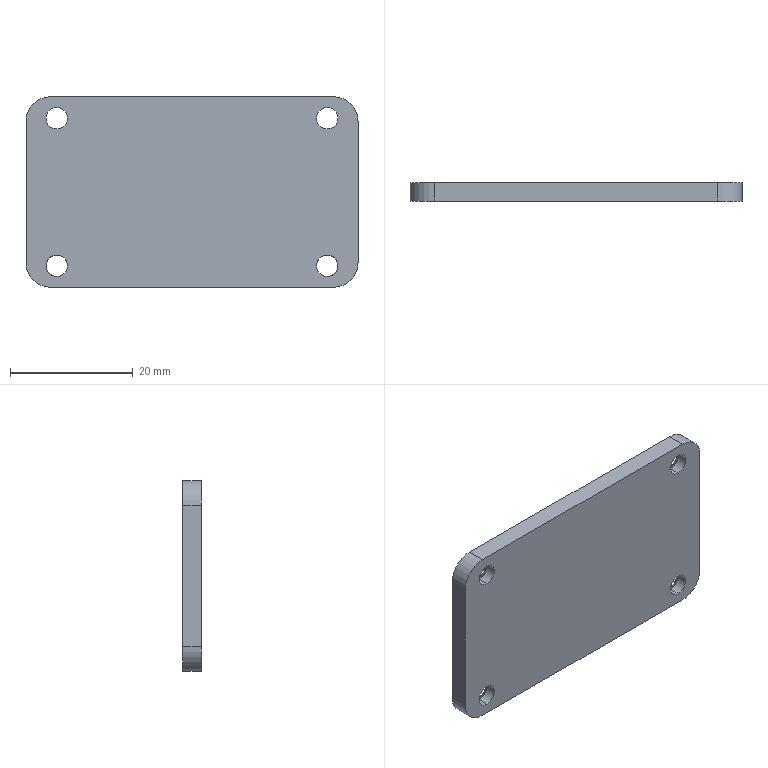Part | STEP file | 1 solid | 26 faces | box 54 x 3 x 31 mm | volume 4823 mm3 | cylinder 12 | cone 8 | plane 6 | commonest cylinder face diameters 3.5 x8 8 x4
STEP:
#1=CARTESIAN_POINT('',(-22.,1.75,13.75));
#2=VERTEX_POINT('',#1);
#3=CARTESIAN_POINT('',(-22.,1.75,10.25));
#4=VERTEX_POINT('',#3);
#5=CARTESIAN_POINT('',(-22.,1.75,12.));
#6=DIRECTION('',(0.,-1.,0.));
#7=DIRECTION('',(0.,0.,-1.));
#8=AXIS2_PLACEMENT_3D('',#5,#6,#7);
#9=CIRCLE('',#8,1.75);
#10=EDGE_CURVE('',#2,#4,#9,.T.);
#11=ORIENTED_EDGE('',*,*,#10,.F.);
#12=CARTESIAN_POINT('',(-22.,0.,13.75));
#13=VERTEX_POINT('',#12);
#14=CARTESIAN_POINT('',(-22.,9.585,13.75));
#15=DIRECTION('',(0.,-1.,0.));
#16=VECTOR('',#15,1000.);
#17=LINE('',#14,#16);
#18=EDGE_CURVE('',#2,#13,#17,.T.);
#19=ORIENTED_EDGE('',*,*,#18,.T.);
#20=CARTESIAN_POINT('',(-22.,0.,10.25));
#21=VERTEX_POINT('',#20);
#22=CARTESIAN_POINT('',(-22.,0.,12.));
#23=DIRECTION('',(0.,1.,0.));
#24=DIRECTION('',(0.,0.,-1.));
#25=AXIS2_PLACEMENT_3D('',#22,#23,#24);
#26=CIRCLE('',#25,1.75);
#27=EDGE_CURVE('',#21,#13,#26,.T.);
#28=ORIENTED_EDGE('',*,*,#27,.F.);
#29=CARTESIAN_POINT('',(-22.,9.585,10.25));
#30=DIRECTION('',(0.,-1.,0.));
#31=VECTOR('',#30,1000.);
#32=LINE('',#29,#31);
#33=EDGE_CURVE('',#4,#21,#32,.T.);
#34=ORIENTED_EDGE('',*,*,#33,.F.);
#35=EDGE_LOOP('',(#11,#19,#28,#34));
#36=FACE_OUTER_BOUND('',#35,.T.);
#37=CARTESIAN_POINT('',(-22.,9.585,12.));
#38=DIRECTION('',(0.,-1.,0.));
#39=DIRECTION('',(0.,0.,-1.));
#40=AXIS2_PLACEMENT_3D('',#37,#38,#39);
#41=CYLINDRICAL_SURFACE('',#40,1.75);
#42=ADVANCED_FACE('',(#36),#41,.F.);
#43=CARTESIAN_POINT('',(-22.,1.75,-10.25));
#44=VERTEX_POINT('',#43);
#45=CARTESIAN_POINT('',(-23.75,1.75,-12.));
#46=VERTEX_POINT('',#45);
#47=CARTESIAN_POINT('',(-22.,1.75,-12.));
#48=DIRECTION('',(0.,-1.,0.));
#49=DIRECTION('',(0.,0.,-1.));
#50=AXIS2_PLACEMENT_3D('',#47,#48,#49);
#51=CIRCLE('',#50,1.75);
#52=EDGE_CURVE('',#44,#46,#51,.T.);
#53=ORIENTED_EDGE('',*,*,#52,.F.);
#54=CARTESIAN_POINT('',(-22.,0.,-10.25));
#55=VERTEX_POINT('',#54);
#56=CARTESIAN_POINT('',(-22.,9.585,-10.25));
#57=DIRECTION('',(0.,-1.,0.));
#58=VECTOR('',#57,1000.);
#59=LINE('',#56,#58);
#60=EDGE_CURVE('',#44,#55,#59,.T.);
#61=ORIENTED_EDGE('',*,*,#60,.T.);
#62=CARTESIAN_POINT('',(-22.,0.,-13.75));
#63=VERTEX_POINT('',#62);
#64=CARTESIAN_POINT('',(-22.,0.,-12.));
#65=DIRECTION('',(0.,1.,0.));
#66=DIRECTION('',(0.,0.,-1.));
#67=AXIS2_PLACEMENT_3D('',#64,#65,#66);
#68=CIRCLE('',#67,1.75);
#69=EDGE_CURVE('',#63,#55,#68,.T.);
#70=ORIENTED_EDGE('',*,*,#69,.F.);
#71=CARTESIAN_POINT('',(-22.,1.75,-13.75));
#72=VERTEX_POINT('',#71);
#73=CARTESIAN_POINT('',(-22.,9.585,-13.75));
#74=DIRECTION('',(0.,-1.,0.));
#75=VECTOR('',#74,1000.);
#76=LINE('',#73,#75);
#77=EDGE_CURVE('',#72,#63,#76,.T.);
#78=ORIENTED_EDGE('',*,*,#77,.F.);
#79=CARTESIAN_POINT('',(-22.,1.75,-12.));
#80=DIRECTION('',(0.,-1.,0.));
#81=DIRECTION('',(0.,0.,-1.));
#82=AXIS2_PLACEMENT_3D('',#79,#80,#81);
#83=CIRCLE('',#82,1.75);
#84=EDGE_CURVE('',#46,#72,#83,.T.);
#85=ORIENTED_EDGE('',*,*,#84,.F.);
#86=EDGE_LOOP('',(#53,#61,#70,#78,#85));
#87=FACE_OUTER_BOUND('',#86,.T.);
#88=CARTESIAN_POINT('',(-22.,9.585,-12.));
#89=DIRECTION('',(0.,-1.,0.));
#90=DIRECTION('',(0.,0.,-1.));
#91=AXIS2_PLACEMENT_3D('',#88,#89,#90);
#92=CYLINDRICAL_SURFACE('',#91,1.75);
#93=ADVANCED_FACE('',(#87),#92,.F.);
#94=CARTESIAN_POINT('',(22.,1.75,-10.25));
#95=VERTEX_POINT('',#94);
#96=CARTESIAN_POINT('',(20.25,1.75,-12.));
#97=VERTEX_POINT('',#96);
#98=CARTESIAN_POINT('',(22.,1.75,-12.));
#99=DIRECTION('',(0.,-1.,0.));
#100=DIRECTION('',(0.,0.,-1.));
#101=AXIS2_PLACEMENT_3D('',#98,#99,#100);
#102=CIRCLE('',#101,1.75);
#103=EDGE_CURVE('',#95,#97,#102,.T.);
#104=ORIENTED_EDGE('',*,*,#103,.F.);
#105=CARTESIAN_POINT('',(22.,0.,-10.25));
#106=VERTEX_POINT('',#105);
#107=CARTESIAN_POINT('',(22.,9.585,-10.25));
#108=DIRECTION('',(0.,-1.,0.));
#109=VECTOR('',#108,1000.);
#110=LINE('',#107,#109);
#111=EDGE_CURVE('',#95,#106,#110,.T.);
#112=ORIENTED_EDGE('',*,*,#111,.T.);
#113=CARTESIAN_POINT('',(22.,0.,-13.75));
#114=VERTEX_POINT('',#113);
#115=CARTESIAN_POINT('',(22.,0.,-12.));
#116=DIRECTION('',(0.,1.,0.));
#117=DIRECTION('',(0.,0.,-1.));
#118=AXIS2_PLACEMENT_3D('',#115,#116,#117);
#119=CIRCLE('',#118,1.75);
#120=EDGE_CURVE('',#114,#106,#119,.T.);
#121=ORIENTED_EDGE('',*,*,#120,.F.);
#122=CARTESIAN_POINT('',(22.,1.75,-13.75));
#123=VERTEX_POINT('',#122);
#124=CARTESIAN_POINT('',(22.,9.585,-13.75));
#125=DIRECTION('',(0.,-1.,0.));
#126=VECTOR('',#125,1000.);
#127=LINE('',#124,#126);
#128=EDGE_CURVE('',#123,#114,#127,.T.);
#129=ORIENTED_EDGE('',*,*,#128,.F.);
#130=CARTESIAN_POINT('',(22.,1.75,-12.));
#131=DIRECTION('',(0.,-1.,0.));
#132=DIRECTION('',(0.,0.,-1.));
#133=AXIS2_PLACEMENT_3D('',#130,#131,#132);
#134=CIRCLE('',#133,1.75);
#135=EDGE_CURVE('',#97,#123,#134,.T.);
#136=ORIENTED_EDGE('',*,*,#135,.F.);
#137=EDGE_LOOP('',(#104,#112,#121,#129,#136));
#138=FACE_OUTER_BOUND('',#137,.T.);
#139=CARTESIAN_POINT('',(22.,9.585,-12.));
#140=DIRECTION('',(0.,-1.,0.));
#141=DIRECTION('',(0.,0.,-1.));
#142=AXIS2_PLACEMENT_3D('',#139,#140,#141);
#143=CYLINDRICAL_SURFACE('',#142,1.75);
#144=ADVANCED_FACE('',(#138),#143,.F.);
#145=CARTESIAN_POINT('',(22.,1.75,13.75));
#146=VERTEX_POINT('',#145);
#147=CARTESIAN_POINT('',(22.,1.75,10.25));
#148=VERTEX_POINT('',#147);
#149=CARTESIAN_POINT('',(22.,1.75,12.));
#150=DIRECTION('',(0.,-1.,0.));
#151=DIRECTION('',(0.,0.,-1.));
#152=AXIS2_PLACEMENT_3D('',#149,#150,#151);
#153=CIRCLE('',#152,1.75);
#154=EDGE_CURVE('',#146,#148,#153,.T.);
#155=ORIENTED_EDGE('',*,*,#154,.F.);
#156=CARTESIAN_POINT('',(22.,0.,13.75));
#157=VERTEX_POINT('',#156);
#158=CARTESIAN_POINT('',(22.,9.585,13.75));
#159=DIRECTION('',(0.,-1.,0.));
#160=VECTOR('',#159,1000.);
#161=LINE('',#158,#160);
#162=EDGE_CURVE('',#146,#157,#161,.T.);
#163=ORIENTED_EDGE('',*,*,#162,.T.);
#164=CARTESIAN_POINT('',(22.,0.,10.25));
#165=VERTEX_POINT('',#164);
#166=CARTESIAN_POINT('',(22.,0.,12.));
#167=DIRECTION('',(0.,1.,0.));
#168=DIRECTION('',(0.,0.,-1.));
#169=AXIS2_PLACEMENT_3D('',#166,#167,#168);
#170=CIRCLE('',#169,1.75);
#171=EDGE_CURVE('',#165,#157,#170,.T.);
#172=ORIENTED_EDGE('',*,*,#171,.F.);
#173=CARTESIAN_POINT('',(22.,9.585,10.25));
#174=DIRECTION('',(0.,-1.,0.));
#175=VECTOR('',#174,1000.);
#176=LINE('',#173,#175);
#177=EDGE_CURVE('',#148,#165,#176,.T.);
#178=ORIENTED_EDGE('',*,*,#177,.F.);
#179=EDGE_LOOP('',(#155,#163,#172,#178));
#180=FACE_OUTER_BOUND('',#179,.T.);
#181=CARTESIAN_POINT('',(22.,9.585,12.));
#182=DIRECTION('',(0.,-1.,0.));
#183=DIRECTION('',(0.,0.,-1.));
#184=AXIS2_PLACEMENT_3D('',#181,#182,#183);
#185=CYLINDRICAL_SURFACE('',#184,1.75);
#186=ADVANCED_FACE('',(#180),#185,.F.);
#187=ORIENTED_EDGE('',*,*,#10,.T.);
#188=CARTESIAN_POINT('',(-22.,3.,9.));
#189=VERTEX_POINT('',#188);
#190=CARTESIAN_POINT('',(-22.,3.,9.));
#191=DIRECTION('',(0.,0.7071,-0.7071));
#192=VECTOR('',#191,1000.);
#193=LINE('',#190,#192);
#194=EDGE_CURVE('',#4,#189,#193,.T.);
#195=ORIENTED_EDGE('',*,*,#194,.T.);
#196=CARTESIAN_POINT('',(-22.,3.,15.));
#197=VERTEX_POINT('',#196);
#198=CARTESIAN_POINT('',(-22.,3.,12.));
#199=DIRECTION('',(0.,-1.,0.));
#200=DIRECTION('',(0.,0.,1.));
#201=AXIS2_PLACEMENT_3D('',#198,#199,#200);
#202=CIRCLE('',#201,3.);
#203=EDGE_CURVE('',#197,#189,#202,.T.);
#204=ORIENTED_EDGE('',*,*,#203,.F.);
#205=CARTESIAN_POINT('',(-22.,3.,15.));
#206=DIRECTION('',(0.,0.7071,0.7071));
#207=VECTOR('',#206,1000.);
#208=LINE('',#205,#207);
#209=EDGE_CURVE('',#2,#197,#208,.T.);
#210=ORIENTED_EDGE('',*,*,#209,.F.);
#211=EDGE_LOOP('',(#187,#195,#204,#210));
#212=FACE_OUTER_BOUND('',#211,.T.);
#213=CARTESIAN_POINT('',(-22.,3.,12.));
#214=DIRECTION('',(0.,1.,0.));
#215=DIRECTION('',(0.,0.,1.));
#216=AXIS2_PLACEMENT_3D('',#213,#214,#215);
#217=CONICAL_SURFACE('',#216,3.,0.7854);
#218=ADVANCED_FACE('',(#212),#217,.F.);
#219=ORIENTED_EDGE('',*,*,#84,.T.);
#220=CARTESIAN_POINT('',(-20.25,1.75,-12.));
#221=VERTEX_POINT('',#220);
#222=CARTESIAN_POINT('',(-22.,1.75,-12.));
#223=DIRECTION('',(0.,-1.,0.));
#224=DIRECTION('',(0.,0.,-1.));
#225=AXIS2_PLACEMENT_3D('',#222,#223,#224);
#226=CIRCLE('',#225,1.75);
#227=EDGE_CURVE('',#72,#221,#226,.T.);
#228=ORIENTED_EDGE('',*,*,#227,.T.);
#229=CARTESIAN_POINT('',(-19.,3.,-12.));
#230=VERTEX_POINT('',#229);
#231=CARTESIAN_POINT('',(-19.,3.,-12.));
#232=DIRECTION('',(0.7071,0.7071,0.));
#233=VECTOR('',#232,1000.);
#234=LINE('',#231,#233);
#235=EDGE_CURVE('',#221,#230,#234,.T.);
#236=ORIENTED_EDGE('',*,*,#235,.T.);
#237=CARTESIAN_POINT('',(-25.,3.,-12.));
#238=VERTEX_POINT('',#237);
#239=CARTESIAN_POINT('',(-22.,3.,-12.));
#240=DIRECTION('',(0.,-1.,0.));
#241=DIRECTION('',(-1.,0.,0.));
#242=AXIS2_PLACEMENT_3D('',#239,#240,#241);
#243=CIRCLE('',#242,3.);
#244=EDGE_CURVE('',#238,#230,#243,.T.);
#245=ORIENTED_EDGE('',*,*,#244,.F.);
#246=CARTESIAN_POINT('',(-25.,3.,-12.));
#247=DIRECTION('',(-0.7071,0.7071,0.));
#248=VECTOR('',#247,1000.);
#249=LINE('',#246,#248);
#250=EDGE_CURVE('',#46,#238,#249,.T.);
#251=ORIENTED_EDGE('',*,*,#250,.F.);
#252=EDGE_LOOP('',(#219,#228,#236,#245,#251));
#253=FACE_OUTER_BOUND('',#252,.T.);
#254=CARTESIAN_POINT('',(-22.,3.,-12.));
#255=DIRECTION('',(0.,1.,0.));
#256=DIRECTION('',(-1.,0.,0.));
#257=AXIS2_PLACEMENT_3D('',#254,#255,#256);
#258=CONICAL_SURFACE('',#257,3.,0.7854);
#259=ADVANCED_FACE('',(#253),#258,.F.);
#260=ORIENTED_EDGE('',*,*,#135,.T.);
#261=CARTESIAN_POINT('',(23.75,1.75,-12.));
#262=VERTEX_POINT('',#261);
#263=CARTESIAN_POINT('',(22.,1.75,-12.));
#264=DIRECTION('',(0.,-1.,0.));
#265=DIRECTION('',(0.,0.,-1.));
#266=AXIS2_PLACEMENT_3D('',#263,#264,#265);
#267=CIRCLE('',#266,1.75);
#268=EDGE_CURVE('',#123,#262,#267,.T.);
#269=ORIENTED_EDGE('',*,*,#268,.T.);
#270=CARTESIAN_POINT('',(25.,3.,-12.));
#271=VERTEX_POINT('',#270);
#272=CARTESIAN_POINT('',(25.,3.,-12.));
#273=DIRECTION('',(0.7071,0.7071,0.));
#274=VECTOR('',#273,1000.);
#275=LINE('',#272,#274);
#276=EDGE_CURVE('',#262,#271,#275,.T.);
#277=ORIENTED_EDGE('',*,*,#276,.T.);
#278=CARTESIAN_POINT('',(19.,3.,-12.));
#279=VERTEX_POINT('',#278);
#280=CARTESIAN_POINT('',(22.,3.,-12.));
#281=DIRECTION('',(0.,-1.,0.));
#282=DIRECTION('',(-1.,0.,0.));
#283=AXIS2_PLACEMENT_3D('',#280,#281,#282);
#284=CIRCLE('',#283,3.);
#285=EDGE_CURVE('',#279,#271,#284,.T.);
#286=ORIENTED_EDGE('',*,*,#285,.F.);
#287=CARTESIAN_POINT('',(19.,3.,-12.));
#288=DIRECTION('',(-0.7071,0.7071,0.));
#289=VECTOR('',#288,1000.);
#290=LINE('',#287,#289);
#291=EDGE_CURVE('',#97,#279,#290,.T.);
#292=ORIENTED_EDGE('',*,*,#291,.F.);
#293=EDGE_LOOP('',(#260,#269,#277,#286,#292));
#294=FACE_OUTER_BOUND('',#293,.T.);
#295=CARTESIAN_POINT('',(22.,3.,-12.));
#296=DIRECTION('',(0.,1.,0.));
#297=DIRECTION('',(-1.,0.,0.));
#298=AXIS2_PLACEMENT_3D('',#295,#296,#297);
#299=CONICAL_SURFACE('',#298,3.,0.7854);
#300=ADVANCED_FACE('',(#294),#299,.F.);
#301=ORIENTED_EDGE('',*,*,#154,.T.);
#302=CARTESIAN_POINT('',(22.,3.,9.));
#303=VERTEX_POINT('',#302);
#304=CARTESIAN_POINT('',(22.,3.,9.));
#305=DIRECTION('',(0.,0.7071,-0.7071));
#306=VECTOR('',#305,1000.);
#307=LINE('',#304,#306);
#308=EDGE_CURVE('',#148,#303,#307,.T.);
#309=ORIENTED_EDGE('',*,*,#308,.T.);
#310=CARTESIAN_POINT('',(22.,3.,15.));
#311=VERTEX_POINT('',#310);
#312=CARTESIAN_POINT('',(22.,3.,12.));
#313=DIRECTION('',(0.,-1.,0.));
#314=DIRECTION('',(0.,0.,1.));
#315=AXIS2_PLACEMENT_3D('',#312,#313,#314);
#316=CIRCLE('',#315,3.);
#317=EDGE_CURVE('',#311,#303,#316,.T.);
#318=ORIENTED_EDGE('',*,*,#317,.F.);
#319=CARTESIAN_POINT('',(22.,3.,15.));
#320=DIRECTION('',(0.,0.7071,0.7071));
#321=VECTOR('',#320,1000.);
#322=LINE('',#319,#321);
#323=EDGE_CURVE('',#146,#311,#322,.T.);
#324=ORIENTED_EDGE('',*,*,#323,.F.);
#325=EDGE_LOOP('',(#301,#309,#318,#324));
#326=FACE_OUTER_BOUND('',#325,.T.);
#327=CARTESIAN_POINT('',(22.,3.,12.));
#328=DIRECTION('',(0.,1.,0.));
#329=DIRECTION('',(0.,0.,1.));
#330=AXIS2_PLACEMENT_3D('',#327,#328,#329);
#331=CONICAL_SURFACE('',#330,3.,0.7854);
#332=ADVANCED_FACE('',(#326),#331,.F.);
#333=CARTESIAN_POINT('',(23.,0.,-15.5));
#334=VERTEX_POINT('',#333);
#335=CARTESIAN_POINT('',(27.,0.,-11.5));
#336=VERTEX_POINT('',#335);
#337=CARTESIAN_POINT('',(23.,0.,-11.5));
#338=DIRECTION('',(0.,-1.,0.));
#339=DIRECTION('',(0.,0.,-1.));
#340=AXIS2_PLACEMENT_3D('',#337,#338,#339);
#341=CIRCLE('',#340,4.);
#342=EDGE_CURVE('',#334,#336,#341,.T.);
#343=ORIENTED_EDGE('',*,*,#342,.T.);
#344=CARTESIAN_POINT('',(27.,0.,11.5));
#345=VERTEX_POINT('',#344);
#346=CARTESIAN_POINT('',(27.,0.,-62.266));
#347=DIRECTION('',(0.,0.,1.));
#348=VECTOR('',#347,1000.);
#349=LINE('',#346,#348);
#350=EDGE_CURVE('',#336,#345,#349,.T.);
#351=ORIENTED_EDGE('',*,*,#350,.T.);
#352=CARTESIAN_POINT('',(23.,0.,15.5));
#353=VERTEX_POINT('',#352);
#354=CARTESIAN_POINT('',(23.,0.,11.5));
#355=DIRECTION('',(0.,-1.,0.));
#356=DIRECTION('',(0.,0.,-1.));
#357=AXIS2_PLACEMENT_3D('',#354,#355,#356);
#358=CIRCLE('',#357,4.);
#359=EDGE_CURVE('',#345,#353,#358,.T.);
#360=ORIENTED_EDGE('',*,*,#359,.T.);
#361=CARTESIAN_POINT('',(-23.,0.,15.5));
#362=VERTEX_POINT('',#361);
#363=CARTESIAN_POINT('',(62.266,0.,15.5));
#364=DIRECTION('',(-1.,0.,0.));
#365=VECTOR('',#364,1000.);
#366=LINE('',#363,#365);
#367=EDGE_CURVE('',#353,#362,#366,.T.);
#368=ORIENTED_EDGE('',*,*,#367,.T.);
#369=CARTESIAN_POINT('',(-27.,0.,11.5));
#370=VERTEX_POINT('',#369);
#371=CARTESIAN_POINT('',(-23.,0.,11.5));
#372=DIRECTION('',(0.,-1.,0.));
#373=DIRECTION('',(0.,0.,-1.));
#374=AXIS2_PLACEMENT_3D('',#371,#372,#373);
#375=CIRCLE('',#374,4.);
#376=EDGE_CURVE('',#362,#370,#375,.T.);
#377=ORIENTED_EDGE('',*,*,#376,.T.);
#378=CARTESIAN_POINT('',(-27.,0.,-11.5));
#379=VERTEX_POINT('',#378);
#380=CARTESIAN_POINT('',(-27.,0.,-62.266));
#381=DIRECTION('',(0.,0.,-1.));
#382=VECTOR('',#381,1000.);
#383=LINE('',#380,#382);
#384=EDGE_CURVE('',#370,#379,#383,.T.);
#385=ORIENTED_EDGE('',*,*,#384,.T.);
#386=CARTESIAN_POINT('',(-23.,0.,-15.5));
#387=VERTEX_POINT('',#386);
#388=CARTESIAN_POINT('',(-23.,0.,-11.5));
#389=DIRECTION('',(0.,-1.,0.));
#390=DIRECTION('',(0.,0.,-1.));
#391=AXIS2_PLACEMENT_3D('',#388,#389,#390);
#392=CIRCLE('',#391,4.);
#393=EDGE_CURVE('',#379,#387,#392,.T.);
#394=ORIENTED_EDGE('',*,*,#393,.T.);
#395=CARTESIAN_POINT('',(62.266,0.,-15.5));
#396=DIRECTION('',(1.,0.,0.));
#397=VECTOR('',#396,1000.);
#398=LINE('',#395,#397);
#399=EDGE_CURVE('',#387,#334,#398,.T.);
#400=ORIENTED_EDGE('',*,*,#399,.T.);
#401=EDGE_LOOP('',(#343,#351,#360,#368,#377,#385,#394,#400));
#402=FACE_OUTER_BOUND('',#401,.T.);
#403=ORIENTED_EDGE('',*,*,#27,.T.);
#404=CARTESIAN_POINT('',(-22.,0.,12.));
#405=DIRECTION('',(0.,1.,0.));
#406=DIRECTION('',(0.,0.,-1.));
#407=AXIS2_PLACEMENT_3D('',#404,#405,#406);
#408=CIRCLE('',#407,1.75);
#409=EDGE_CURVE('',#13,#21,#408,.T.);
#410=ORIENTED_EDGE('',*,*,#409,.T.);
#411=EDGE_LOOP('',(#403,#410));
#412=FACE_BOUND('',#411,.T.);
#413=ORIENTED_EDGE('',*,*,#69,.T.);
#414=CARTESIAN_POINT('',(-22.,0.,-12.));
#415=DIRECTION('',(0.,1.,0.));
#416=DIRECTION('',(0.,0.,-1.));
#417=AXIS2_PLACEMENT_3D('',#414,#415,#416);
#418=CIRCLE('',#417,1.75);
#419=EDGE_CURVE('',#55,#63,#418,.T.);
#420=ORIENTED_EDGE('',*,*,#419,.T.);
#421=EDGE_LOOP('',(#413,#420));
#422=FACE_BOUND('',#421,.T.);
#423=ORIENTED_EDGE('',*,*,#120,.T.);
#424=CARTESIAN_POINT('',(22.,0.,-12.));
#425=DIRECTION('',(0.,1.,0.));
#426=DIRECTION('',(0.,0.,-1.));
#427=AXIS2_PLACEMENT_3D('',#424,#425,#426);
#428=CIRCLE('',#427,1.75);
#429=EDGE_CURVE('',#106,#114,#428,.T.);
#430=ORIENTED_EDGE('',*,*,#429,.T.);
#431=EDGE_LOOP('',(#423,#430));
#432=FACE_BOUND('',#431,.T.);
#433=ORIENTED_EDGE('',*,*,#171,.T.);
#434=CARTESIAN_POINT('',(22.,0.,12.));
#435=DIRECTION('',(0.,1.,0.));
#436=DIRECTION('',(0.,0.,-1.));
#437=AXIS2_PLACEMENT_3D('',#434,#435,#436);
#438=CIRCLE('',#437,1.75);
#439=EDGE_CURVE('',#157,#165,#438,.T.);
#440=ORIENTED_EDGE('',*,*,#439,.T.);
#441=EDGE_LOOP('',(#433,#440));
#442=FACE_BOUND('',#441,.T.);
#443=CARTESIAN_POINT('',(62.266,0.,-62.266));
#444=DIRECTION('',(0.,-1.,0.));
#445=DIRECTION('',(0.,0.,-1.));
#446=AXIS2_PLACEMENT_3D('',#443,#444,#445);
#447=PLANE('',#446);
#448=ADVANCED_FACE('',(#402,#412,#422,#432,#442),#447,.T.);
#449=CARTESIAN_POINT('',(27.,3.,-11.5));
#450=VERTEX_POINT('',#449);
#451=CARTESIAN_POINT('',(27.,41.767,-11.5));
#452=DIRECTION('',(0.,1.,0.));
#453=VECTOR('',#452,1000.);
#454=LINE('',#451,#453);
#455=EDGE_CURVE('',#336,#450,#454,.T.);
#456=ORIENTED_EDGE('',*,*,#455,.T.);
#457=CARTESIAN_POINT('',(27.,3.,11.5));
#458=VERTEX_POINT('',#457);
#459=CARTESIAN_POINT('',(27.,3.,-54.267));
#460=DIRECTION('',(0.,0.,1.));
#461=VECTOR('',#460,1000.);
#462=LINE('',#459,#461);
#463=EDGE_CURVE('',#450,#458,#462,.T.);
#464=ORIENTED_EDGE('',*,*,#463,.T.);
#465=CARTESIAN_POINT('',(27.,41.767,11.5));
#466=DIRECTION('',(0.,-1.,0.));
#467=VECTOR('',#466,1000.);
#468=LINE('',#465,#467);
#469=EDGE_CURVE('',#458,#345,#468,.T.);
#470=ORIENTED_EDGE('',*,*,#469,.T.);
#471=ORIENTED_EDGE('',*,*,#350,.F.);
#472=EDGE_LOOP('',(#456,#464,#470,#471));
#473=FACE_OUTER_BOUND('',#472,.T.);
#474=CARTESIAN_POINT('',(27.,41.767,-54.267));
#475=DIRECTION('',(1.,0.,0.));
#476=DIRECTION('',(0.,1.,0.));
#477=AXIS2_PLACEMENT_3D('',#474,#475,#476);
#478=PLANE('',#477);
#479=ADVANCED_FACE('',(#473),#478,.T.);
#480=ORIENTED_EDGE('',*,*,#342,.F.);
#481=CARTESIAN_POINT('',(23.,3.,-15.5));
#482=VERTEX_POINT('',#481);
#483=CARTESIAN_POINT('',(23.,12.605,-15.5));
#484=DIRECTION('',(0.,1.,0.));
#485=VECTOR('',#484,1000.);
#486=LINE('',#483,#485);
#487=EDGE_CURVE('',#334,#482,#486,.T.);
#488=ORIENTED_EDGE('',*,*,#487,.T.);
#489=CARTESIAN_POINT('',(23.,3.,-11.5));
#490=DIRECTION('',(0.,-1.,0.));
#491=DIRECTION('',(0.,0.,-1.));
#492=AXIS2_PLACEMENT_3D('',#489,#490,#491);
#493=CIRCLE('',#492,4.);
#494=EDGE_CURVE('',#482,#450,#493,.T.);
#495=ORIENTED_EDGE('',*,*,#494,.T.);
#496=ORIENTED_EDGE('',*,*,#455,.F.);
#497=EDGE_LOOP('',(#480,#488,#495,#496));
#498=FACE_OUTER_BOUND('',#497,.T.);
#499=CARTESIAN_POINT('',(23.,12.605,-11.5));
#500=DIRECTION('',(0.,-1.,0.));
#501=DIRECTION('',(0.,0.,-1.));
#502=AXIS2_PLACEMENT_3D('',#499,#500,#501);
#503=CYLINDRICAL_SURFACE('',#502,4.);
#504=ADVANCED_FACE('',(#498),#503,.T.);
#505=CARTESIAN_POINT('',(-23.,3.,-15.5));
#506=VERTEX_POINT('',#505);
#507=CARTESIAN_POINT('',(-23.,76.139,-15.5));
#508=DIRECTION('',(0.,1.,0.));
#509=VECTOR('',#508,1000.);
#510=LINE('',#507,#509);
#511=EDGE_CURVE('',#387,#506,#510,.T.);
#512=ORIENTED_EDGE('',*,*,#511,.T.);
#513=CARTESIAN_POINT('',(-100.139,3.,-15.5));
#514=DIRECTION('',(1.,0.,0.));
#515=VECTOR('',#514,1000.);
#516=LINE('',#513,#515);
#517=EDGE_CURVE('',#506,#482,#516,.T.);
#518=ORIENTED_EDGE('',*,*,#517,.T.);
#519=ORIENTED_EDGE('',*,*,#487,.F.);
#520=ORIENTED_EDGE('',*,*,#399,.F.);
#521=EDGE_LOOP('',(#512,#518,#519,#520));
#522=FACE_OUTER_BOUND('',#521,.T.);
#523=CARTESIAN_POINT('',(-100.139,76.139,-15.5));
#524=DIRECTION('',(0.,0.,-1.));
#525=DIRECTION('',(0.,-1.,0.));
#526=AXIS2_PLACEMENT_3D('',#523,#524,#525);
#527=PLANE('',#526);
#528=ADVANCED_FACE('',(#522),#527,.T.);
#529=ORIENTED_EDGE('',*,*,#393,.F.);
#530=CARTESIAN_POINT('',(-27.,3.,-11.5));
#531=VERTEX_POINT('',#530);
#532=CARTESIAN_POINT('',(-27.,12.605,-11.5));
#533=DIRECTION('',(0.,1.,0.));
#534=VECTOR('',#533,1000.);
#535=LINE('',#532,#534);
#536=EDGE_CURVE('',#379,#531,#535,.T.);
#537=ORIENTED_EDGE('',*,*,#536,.T.);
#538=CARTESIAN_POINT('',(-23.,3.,-11.5));
#539=DIRECTION('',(0.,-1.,0.));
#540=DIRECTION('',(0.,0.,-1.));
#541=AXIS2_PLACEMENT_3D('',#538,#539,#540);
#542=CIRCLE('',#541,4.);
#543=EDGE_CURVE('',#531,#506,#542,.T.);
#544=ORIENTED_EDGE('',*,*,#543,.T.);
#545=ORIENTED_EDGE('',*,*,#511,.F.);
#546=EDGE_LOOP('',(#529,#537,#544,#545));
#547=FACE_OUTER_BOUND('',#546,.T.);
#548=CARTESIAN_POINT('',(-23.,12.605,-11.5));
#549=DIRECTION('',(0.,-1.,0.));
#550=DIRECTION('',(0.,0.,-1.));
#551=AXIS2_PLACEMENT_3D('',#548,#549,#550);
#552=CYLINDRICAL_SURFACE('',#551,4.);
#553=ADVANCED_FACE('',(#547),#552,.T.);
#554=CARTESIAN_POINT('',(-27.,3.,11.5));
#555=VERTEX_POINT('',#554);
#556=CARTESIAN_POINT('',(-27.,41.767,11.5));
#557=DIRECTION('',(0.,1.,0.));
#558=VECTOR('',#557,1000.);
#559=LINE('',#556,#558);
#560=EDGE_CURVE('',#370,#555,#559,.T.);
#561=ORIENTED_EDGE('',*,*,#560,.T.);
#562=CARTESIAN_POINT('',(-27.,3.,23.267));
#563=DIRECTION('',(0.,0.,-1.));
#564=VECTOR('',#563,1000.);
#565=LINE('',#562,#564);
#566=EDGE_CURVE('',#555,#531,#565,.T.);
#567=ORIENTED_EDGE('',*,*,#566,.T.);
#568=ORIENTED_EDGE('',*,*,#536,.F.);
#569=ORIENTED_EDGE('',*,*,#384,.F.);
#570=EDGE_LOOP('',(#561,#567,#568,#569));
#571=FACE_OUTER_BOUND('',#570,.T.);
#572=CARTESIAN_POINT('',(-27.,41.767,23.267));
#573=DIRECTION('',(-1.,0.,0.));
#574=DIRECTION('',(0.,0.,1.));
#575=AXIS2_PLACEMENT_3D('',#572,#573,#574);
#576=PLANE('',#575);
#577=ADVANCED_FACE('',(#571),#576,.T.);
#578=ORIENTED_EDGE('',*,*,#376,.F.);
#579=CARTESIAN_POINT('',(-23.,3.,15.5));
#580=VERTEX_POINT('',#579);
#581=CARTESIAN_POINT('',(-23.,12.605,15.5));
#582=DIRECTION('',(0.,1.,0.));
#583=VECTOR('',#582,1000.);
#584=LINE('',#581,#583);
#585=EDGE_CURVE('',#362,#580,#584,.T.);
#586=ORIENTED_EDGE('',*,*,#585,.T.);
#587=CARTESIAN_POINT('',(-23.,3.,11.5));
#588=DIRECTION('',(0.,-1.,0.));
#589=DIRECTION('',(0.,0.,-1.));
#590=AXIS2_PLACEMENT_3D('',#587,#588,#589);
#591=CIRCLE('',#590,4.);
#592=EDGE_CURVE('',#580,#555,#591,.T.);
#593=ORIENTED_EDGE('',*,*,#592,.T.);
#594=ORIENTED_EDGE('',*,*,#560,.F.);
#595=EDGE_LOOP('',(#578,#586,#593,#594));
#596=FACE_OUTER_BOUND('',#595,.T.);
#597=CARTESIAN_POINT('',(-23.,12.605,11.5));
#598=DIRECTION('',(0.,-1.,0.));
#599=DIRECTION('',(0.,0.,-1.));
#600=AXIS2_PLACEMENT_3D('',#597,#598,#599);
#601=CYLINDRICAL_SURFACE('',#600,4.);
#602=ADVANCED_FACE('',(#596),#601,.T.);
#603=ORIENTED_EDGE('',*,*,#585,.F.);
#604=ORIENTED_EDGE('',*,*,#367,.F.);
#605=CARTESIAN_POINT('',(23.,3.,15.5));
#606=VERTEX_POINT('',#605);
#607=CARTESIAN_POINT('',(23.,76.139,15.5));
#608=DIRECTION('',(0.,1.,0.));
#609=VECTOR('',#608,1000.);
#610=LINE('',#607,#609);
#611=EDGE_CURVE('',#353,#606,#610,.T.);
#612=ORIENTED_EDGE('',*,*,#611,.T.);
#613=CARTESIAN_POINT('',(46.139,3.,15.5));
#614=DIRECTION('',(-1.,0.,0.));
#615=VECTOR('',#614,1000.);
#616=LINE('',#613,#615);
#617=EDGE_CURVE('',#606,#580,#616,.T.);
#618=ORIENTED_EDGE('',*,*,#617,.T.);
#619=EDGE_LOOP('',(#603,#604,#612,#618));
#620=FACE_OUTER_BOUND('',#619,.T.);
#621=CARTESIAN_POINT('',(46.139,76.139,15.5));
#622=DIRECTION('',(0.,0.,1.));
#623=DIRECTION('',(1.,0.,0.));
#624=AXIS2_PLACEMENT_3D('',#621,#622,#623);
#625=PLANE('',#624);
#626=ADVANCED_FACE('',(#620),#625,.T.);
#627=ORIENTED_EDGE('',*,*,#359,.F.);
#628=ORIENTED_EDGE('',*,*,#469,.F.);
#629=CARTESIAN_POINT('',(23.,3.,11.5));
#630=DIRECTION('',(0.,-1.,0.));
#631=DIRECTION('',(0.,0.,-1.));
#632=AXIS2_PLACEMENT_3D('',#629,#630,#631);
#633=CIRCLE('',#632,4.);
#634=EDGE_CURVE('',#458,#606,#633,.T.);
#635=ORIENTED_EDGE('',*,*,#634,.T.);
#636=ORIENTED_EDGE('',*,*,#611,.F.);
#637=EDGE_LOOP('',(#627,#628,#635,#636));
#638=FACE_OUTER_BOUND('',#637,.T.);
#639=CARTESIAN_POINT('',(23.,12.605,11.5));
#640=DIRECTION('',(0.,-1.,0.));
#641=DIRECTION('',(0.,0.,-1.));
#642=AXIS2_PLACEMENT_3D('',#639,#640,#641);
#643=CYLINDRICAL_SURFACE('',#642,4.);
#644=ADVANCED_FACE('',(#638),#643,.T.);
#645=ORIENTED_EDGE('',*,*,#18,.F.);
#646=CARTESIAN_POINT('',(-22.,1.75,12.));
#647=DIRECTION('',(0.,-1.,0.));
#648=DIRECTION('',(0.,0.,-1.));
#649=AXIS2_PLACEMENT_3D('',#646,#647,#648);
#650=CIRCLE('',#649,1.75);
#651=EDGE_CURVE('',#4,#2,#650,.T.);
#652=ORIENTED_EDGE('',*,*,#651,.F.);
#653=ORIENTED_EDGE('',*,*,#33,.T.);
#654=ORIENTED_EDGE('',*,*,#409,.F.);
#655=EDGE_LOOP('',(#645,#652,#653,#654));
#656=FACE_OUTER_BOUND('',#655,.T.);
#657=CARTESIAN_POINT('',(-22.,9.585,12.));
#658=DIRECTION('',(0.,-1.,0.));
#659=DIRECTION('',(0.,0.,-1.));
#660=AXIS2_PLACEMENT_3D('',#657,#658,#659);
#661=CYLINDRICAL_SURFACE('',#660,1.75);
#662=ADVANCED_FACE('',(#656),#661,.F.);
#663=ORIENTED_EDGE('',*,*,#60,.F.);
#664=CARTESIAN_POINT('',(-22.,1.75,-12.));
#665=DIRECTION('',(0.,-1.,0.));
#666=DIRECTION('',(0.,0.,-1.));
#667=AXIS2_PLACEMENT_3D('',#664,#665,#666);
#668=CIRCLE('',#667,1.75);
#669=EDGE_CURVE('',#221,#44,#668,.T.);
#670=ORIENTED_EDGE('',*,*,#669,.F.);
#671=ORIENTED_EDGE('',*,*,#227,.F.);
#672=ORIENTED_EDGE('',*,*,#77,.T.);
#673=ORIENTED_EDGE('',*,*,#419,.F.);
#674=EDGE_LOOP('',(#663,#670,#671,#672,#673));
#675=FACE_OUTER_BOUND('',#674,.T.);
#676=CARTESIAN_POINT('',(-22.,9.585,-12.));
#677=DIRECTION('',(0.,-1.,0.));
#678=DIRECTION('',(0.,0.,-1.));
#679=AXIS2_PLACEMENT_3D('',#676,#677,#678);
#680=CYLINDRICAL_SURFACE('',#679,1.75);
#681=ADVANCED_FACE('',(#675),#680,.F.);
#682=ORIENTED_EDGE('',*,*,#111,.F.);
#683=CARTESIAN_POINT('',(22.,1.75,-12.));
#684=DIRECTION('',(0.,-1.,0.));
#685=DIRECTION('',(0.,0.,-1.));
#686=AXIS2_PLACEMENT_3D('',#683,#684,#685);
#687=CIRCLE('',#686,1.75);
#688=EDGE_CURVE('',#262,#95,#687,.T.);
#689=ORIENTED_EDGE('',*,*,#688,.F.);
#690=ORIENTED_EDGE('',*,*,#268,.F.);
#691=ORIENTED_EDGE('',*,*,#128,.T.);
#692=ORIENTED_EDGE('',*,*,#429,.F.);
#693=EDGE_LOOP('',(#682,#689,#690,#691,#692));
#694=FACE_OUTER_BOUND('',#693,.T.);
#695=CARTESIAN_POINT('',(22.,9.585,-12.));
#696=DIRECTION('',(0.,-1.,0.));
#697=DIRECTION('',(0.,0.,-1.));
#698=AXIS2_PLACEMENT_3D('',#695,#696,#697);
#699=CYLINDRICAL_SURFACE('',#698,1.75);
#700=ADVANCED_FACE('',(#694),#699,.F.);
#701=ORIENTED_EDGE('',*,*,#162,.F.);
#702=CARTESIAN_POINT('',(22.,1.75,12.));
#703=DIRECTION('',(0.,-1.,0.));
#704=DIRECTION('',(0.,0.,-1.));
#705=AXIS2_PLACEMENT_3D('',#702,#703,#704);
#706=CIRCLE('',#705,1.75);
#707=EDGE_CURVE('',#148,#146,#706,.T.);
#708=ORIENTED_EDGE('',*,*,#707,.F.);
#709=ORIENTED_EDGE('',*,*,#177,.T.);
#710=ORIENTED_EDGE('',*,*,#439,.F.);
#711=EDGE_LOOP('',(#701,#708,#709,#710));
#712=FACE_OUTER_BOUND('',#711,.T.);
#713=CARTESIAN_POINT('',(22.,9.585,12.));
#714=DIRECTION('',(0.,-1.,0.));
#715=DIRECTION('',(0.,0.,-1.));
#716=AXIS2_PLACEMENT_3D('',#713,#714,#715);
#717=CYLINDRICAL_SURFACE('',#716,1.75);
#718=ADVANCED_FACE('',(#712),#717,.F.);
#719=ORIENTED_EDGE('',*,*,#617,.F.);
#720=ORIENTED_EDGE('',*,*,#634,.F.);
#721=ORIENTED_EDGE('',*,*,#463,.F.);
#722=ORIENTED_EDGE('',*,*,#494,.F.);
#723=ORIENTED_EDGE('',*,*,#517,.F.);
#724=ORIENTED_EDGE('',*,*,#543,.F.);
#725=ORIENTED_EDGE('',*,*,#566,.F.);
#726=ORIENTED_EDGE('',*,*,#592,.F.);
#727=EDGE_LOOP('',(#719,#720,#721,#722,#723,#724,#725,#726));
#728=FACE_OUTER_BOUND('',#727,.T.);
#729=ORIENTED_EDGE('',*,*,#203,.T.);
#730=CARTESIAN_POINT('',(-22.,3.,12.));
#731=DIRECTION('',(0.,-1.,0.));
#732=DIRECTION('',(0.,0.,1.));
#733=AXIS2_PLACEMENT_3D('',#730,#731,#732);
#734=CIRCLE('',#733,3.);
#735=EDGE_CURVE('',#189,#197,#734,.T.);
#736=ORIENTED_EDGE('',*,*,#735,.T.);
#737=EDGE_LOOP('',(#729,#736));
#738=FACE_BOUND('',#737,.T.);
#739=ORIENTED_EDGE('',*,*,#317,.T.);
#740=CARTESIAN_POINT('',(22.,3.,12.));
#741=DIRECTION('',(0.,-1.,0.));
#742=DIRECTION('',(0.,0.,1.));
#743=AXIS2_PLACEMENT_3D('',#740,#741,#742);
#744=CIRCLE('',#743,3.);
#745=EDGE_CURVE('',#303,#311,#744,.T.);
#746=ORIENTED_EDGE('',*,*,#745,.T.);
#747=EDGE_LOOP('',(#739,#746));
#748=FACE_BOUND('',#747,.T.);
#749=ORIENTED_EDGE('',*,*,#285,.T.);
#750=CARTESIAN_POINT('',(22.,3.,-12.));
#751=DIRECTION('',(0.,-1.,0.));
#752=DIRECTION('',(-1.,0.,0.));
#753=AXIS2_PLACEMENT_3D('',#750,#751,#752);
#754=CIRCLE('',#753,3.);
#755=EDGE_CURVE('',#271,#279,#754,.T.);
#756=ORIENTED_EDGE('',*,*,#755,.T.);
#757=EDGE_LOOP('',(#749,#756));
#758=FACE_BOUND('',#757,.T.);
#759=ORIENTED_EDGE('',*,*,#244,.T.);
#760=CARTESIAN_POINT('',(-22.,3.,-12.));
#761=DIRECTION('',(0.,-1.,0.));
#762=DIRECTION('',(-1.,0.,0.));
#763=AXIS2_PLACEMENT_3D('',#760,#761,#762);
#764=CIRCLE('',#763,3.);
#765=EDGE_CURVE('',#230,#238,#764,.T.);
#766=ORIENTED_EDGE('',*,*,#765,.T.);
#767=EDGE_LOOP('',(#759,#766));
#768=FACE_BOUND('',#767,.T.);
#769=CARTESIAN_POINT('',(-62.266,3.,-62.266));
#770=DIRECTION('',(0.,1.,0.));
#771=DIRECTION('',(1.,0.,0.));
#772=AXIS2_PLACEMENT_3D('',#769,#770,#771);
#773=PLANE('',#772);
#774=ADVANCED_FACE('',(#728,#738,#748,#758,#768),#773,.T.);
#775=ORIENTED_EDGE('',*,*,#194,.F.);
#776=ORIENTED_EDGE('',*,*,#651,.T.);
#777=ORIENTED_EDGE('',*,*,#209,.T.);
#778=ORIENTED_EDGE('',*,*,#735,.F.);
#779=EDGE_LOOP('',(#775,#776,#777,#778));
#780=FACE_OUTER_BOUND('',#779,.T.);
#781=CARTESIAN_POINT('',(-22.,3.,12.));
#782=DIRECTION('',(0.,1.,0.));
#783=DIRECTION('',(0.,0.,1.));
#784=AXIS2_PLACEMENT_3D('',#781,#782,#783);
#785=CONICAL_SURFACE('',#784,3.,0.7854);
#786=ADVANCED_FACE('',(#780),#785,.F.);
#787=ORIENTED_EDGE('',*,*,#235,.F.);
#788=ORIENTED_EDGE('',*,*,#669,.T.);
#789=ORIENTED_EDGE('',*,*,#52,.T.);
#790=ORIENTED_EDGE('',*,*,#250,.T.);
#791=ORIENTED_EDGE('',*,*,#765,.F.);
#792=EDGE_LOOP('',(#787,#788,#789,#790,#791));
#793=FACE_OUTER_BOUND('',#792,.T.);
#794=CARTESIAN_POINT('',(-22.,3.,-12.));
#795=DIRECTION('',(0.,1.,0.));
#796=DIRECTION('',(-1.,0.,0.));
#797=AXIS2_PLACEMENT_3D('',#794,#795,#796);
#798=CONICAL_SURFACE('',#797,3.,0.7854);
#799=ADVANCED_FACE('',(#793),#798,.F.);
#800=ORIENTED_EDGE('',*,*,#276,.F.);
#801=ORIENTED_EDGE('',*,*,#688,.T.);
#802=ORIENTED_EDGE('',*,*,#103,.T.);
#803=ORIENTED_EDGE('',*,*,#291,.T.);
#804=ORIENTED_EDGE('',*,*,#755,.F.);
#805=EDGE_LOOP('',(#800,#801,#802,#803,#804));
#806=FACE_OUTER_BOUND('',#805,.T.);
#807=CARTESIAN_POINT('',(22.,3.,-12.));
#808=DIRECTION('',(0.,1.,0.));
#809=DIRECTION('',(-1.,0.,0.));
#810=AXIS2_PLACEMENT_3D('',#807,#808,#809);
#811=CONICAL_SURFACE('',#810,3.,0.7854);
#812=ADVANCED_FACE('',(#806),#811,.F.);
#813=ORIENTED_EDGE('',*,*,#308,.F.);
#814=ORIENTED_EDGE('',*,*,#707,.T.);
#815=ORIENTED_EDGE('',*,*,#323,.T.);
#816=ORIENTED_EDGE('',*,*,#745,.F.);
#817=EDGE_LOOP('',(#813,#814,#815,#816));
#818=FACE_OUTER_BOUND('',#817,.T.);
#819=CARTESIAN_POINT('',(22.,3.,12.));
#820=DIRECTION('',(0.,1.,0.));
#821=DIRECTION('',(0.,0.,1.));
#822=AXIS2_PLACEMENT_3D('',#819,#820,#821);
#823=CONICAL_SURFACE('',#822,3.,0.7854);
#824=ADVANCED_FACE('',(#818),#823,.F.);
#825=CLOSED_SHELL('',(#42,#93,#144,#186,#218,#259,#300,#332,#448,#479,#504,#528,#553,#577,#602,#626,#644,#662,#681,#700,#718,#774,#786,#799,#812,#824));
#826=MANIFOLD_SOLID_BREP('',#825);
#827=CARTESIAN_POINT('',(0.,0.,0.));
#828=DIRECTION('',(0.,0.,1.));
#829=DIRECTION('',(1.,0.,0.));
#830=AXIS2_PLACEMENT_3D('',#827,#828,#829);
#831=(LENGTH_UNIT()NAMED_UNIT(*)SI_UNIT(.MILLI.,.METRE.));
#832=UNCERTAINTY_MEASURE_WITH_UNIT(LENGTH_MEASURE(0.00001),#831,'','');
#833=(NAMED_UNIT(*)PLANE_ANGLE_UNIT()SI_UNIT($,.RADIAN.));
#834=(NAMED_UNIT(*)SI_UNIT($,.STERADIAN.)SOLID_ANGLE_UNIT());
#835=(GEOMETRIC_REPRESENTATION_CONTEXT(3)GLOBAL_UNCERTAINTY_ASSIGNED_CONTEXT((#832))GLOBAL_UNIT_ASSIGNED_CONTEXT((#831,#833,#834))REPRESENTATION_CONTEXT('',''));
#836=ADVANCED_BREP_SHAPE_REPRESENTATION('',(#826,#830),#835);